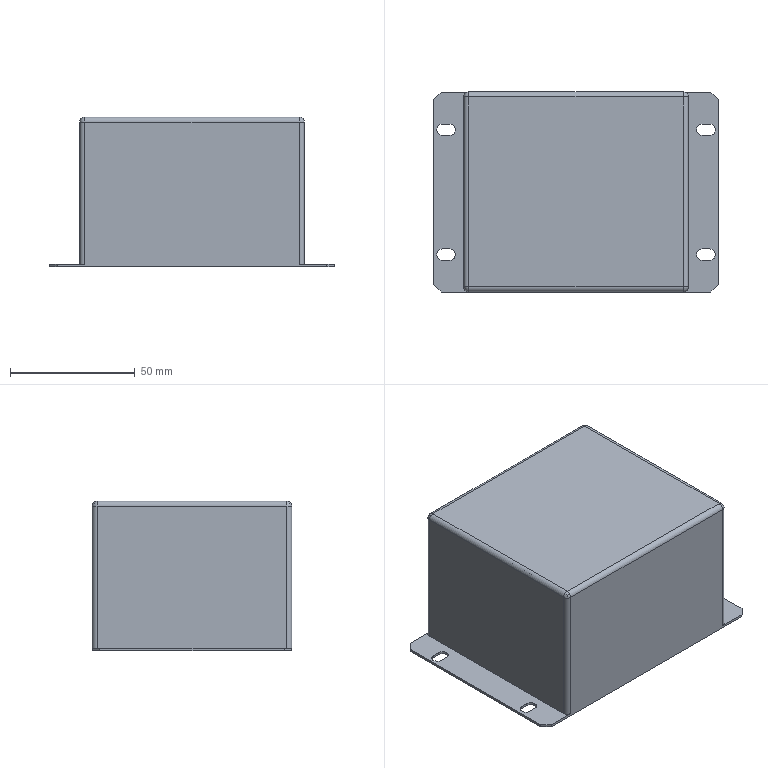Part | STEP file | 11-XJX-00311 | 1 solid | 51 faces | box 114 x 80 x 60 mm | volume 28319 mm3 | plane 27 | cylinder 20 | sphere 4 | commonest cylinder face diameters 4.5 x12 4 x8
STEP:
#1=CARTESIAN_POINT('',(55.75,-25.,0.));
#2=VERTEX_POINT('',#1);
#3=CARTESIAN_POINT('',(53.5,-22.75,0.));
#4=VERTEX_POINT('',#3);
#5=CARTESIAN_POINT('',(53.5,-25.,0.));
#6=DIRECTION('',(0.,0.,1.));
#7=DIRECTION('',(-1.,0.,0.));
#8=AXIS2_PLACEMENT_3D('',#5,#6,#7);
#9=CIRCLE('',#8,2.25);
#10=EDGE_CURVE('',#2,#4,#9,.T.);
#11=ORIENTED_EDGE('',*,*,#10,.F.);
#12=CARTESIAN_POINT('',(55.75,-25.,1.));
#13=VERTEX_POINT('',#12);
#14=CARTESIAN_POINT('',(55.75,-25.,0.));
#15=DIRECTION('',(0.,0.,1.));
#16=VECTOR('',#15,1000.);
#17=LINE('',#14,#16);
#18=EDGE_CURVE('',#2,#13,#17,.T.);
#19=ORIENTED_EDGE('',*,*,#18,.T.);
#20=CARTESIAN_POINT('',(53.5,-22.75,1.));
#21=VERTEX_POINT('',#20);
#22=CARTESIAN_POINT('',(53.5,-25.,1.));
#23=DIRECTION('',(0.,0.,1.));
#24=DIRECTION('',(-1.,0.,0.));
#25=AXIS2_PLACEMENT_3D('',#22,#23,#24);
#26=CIRCLE('',#25,2.25);
#27=EDGE_CURVE('',#13,#21,#26,.T.);
#28=ORIENTED_EDGE('',*,*,#27,.T.);
#29=CARTESIAN_POINT('',(53.5,-22.75,0.));
#30=DIRECTION('',(0.,0.,1.));
#31=VECTOR('',#30,1000.);
#32=LINE('',#29,#31);
#33=EDGE_CURVE('',#4,#21,#32,.T.);
#34=ORIENTED_EDGE('',*,*,#33,.F.);
#35=EDGE_LOOP('',(#11,#19,#28,#34));
#36=FACE_OUTER_BOUND('',#35,.T.);
#37=CARTESIAN_POINT('',(53.5,-25.,0.));
#38=DIRECTION('',(0.,0.,1.));
#39=DIRECTION('',(1.,0.,0.));
#40=AXIS2_PLACEMENT_3D('',#37,#38,#39);
#41=CYLINDRICAL_SURFACE('',#40,2.25);
#42=ADVANCED_FACE('',(#36),#41,.F.);
#43=CARTESIAN_POINT('',(-48.25,25.,0.));
#44=VERTEX_POINT('',#43);
#45=CARTESIAN_POINT('',(-50.5,27.25,0.));
#46=VERTEX_POINT('',#45);
#47=CARTESIAN_POINT('',(-50.5,25.,0.));
#48=DIRECTION('',(0.,0.,1.));
#49=DIRECTION('',(-1.,0.,0.));
#50=AXIS2_PLACEMENT_3D('',#47,#48,#49);
#51=CIRCLE('',#50,2.25);
#52=EDGE_CURVE('',#44,#46,#51,.T.);
#53=ORIENTED_EDGE('',*,*,#52,.F.);
#54=CARTESIAN_POINT('',(-48.25,25.,1.));
#55=VERTEX_POINT('',#54);
#56=CARTESIAN_POINT('',(-48.25,25.,0.));
#57=DIRECTION('',(0.,0.,1.));
#58=VECTOR('',#57,1000.);
#59=LINE('',#56,#58);
#60=EDGE_CURVE('',#44,#55,#59,.T.);
#61=ORIENTED_EDGE('',*,*,#60,.T.);
#62=CARTESIAN_POINT('',(-50.5,27.25,1.));
#63=VERTEX_POINT('',#62);
#64=CARTESIAN_POINT('',(-50.5,25.,1.));
#65=DIRECTION('',(0.,0.,1.));
#66=DIRECTION('',(-1.,0.,0.));
#67=AXIS2_PLACEMENT_3D('',#64,#65,#66);
#68=CIRCLE('',#67,2.25);
#69=EDGE_CURVE('',#55,#63,#68,.T.);
#70=ORIENTED_EDGE('',*,*,#69,.T.);
#71=CARTESIAN_POINT('',(-50.5,27.25,0.));
#72=DIRECTION('',(0.,0.,1.));
#73=VECTOR('',#72,1000.);
#74=LINE('',#71,#73);
#75=EDGE_CURVE('',#46,#63,#74,.T.);
#76=ORIENTED_EDGE('',*,*,#75,.F.);
#77=EDGE_LOOP('',(#53,#61,#70,#76));
#78=FACE_OUTER_BOUND('',#77,.T.);
#79=CARTESIAN_POINT('',(-50.5,25.,0.));
#80=DIRECTION('',(0.,0.,1.));
#81=DIRECTION('',(1.,0.,0.));
#82=AXIS2_PLACEMENT_3D('',#79,#80,#81);
#83=CYLINDRICAL_SURFACE('',#82,2.25);
#84=ADVANCED_FACE('',(#78),#83,.F.);
#85=CARTESIAN_POINT('',(-48.25,-25.,0.));
#86=VERTEX_POINT('',#85);
#87=CARTESIAN_POINT('',(-50.5,-22.75,0.));
#88=VERTEX_POINT('',#87);
#89=CARTESIAN_POINT('',(-50.5,-25.,0.));
#90=DIRECTION('',(0.,0.,1.));
#91=DIRECTION('',(1.,0.,0.));
#92=AXIS2_PLACEMENT_3D('',#89,#90,#91);
#93=CIRCLE('',#92,2.25);
#94=EDGE_CURVE('',#86,#88,#93,.T.);
#95=ORIENTED_EDGE('',*,*,#94,.F.);
#96=CARTESIAN_POINT('',(-48.25,-25.,1.));
#97=VERTEX_POINT('',#96);
#98=CARTESIAN_POINT('',(-48.25,-25.,0.));
#99=DIRECTION('',(0.,0.,1.));
#100=VECTOR('',#99,1000.);
#101=LINE('',#98,#100);
#102=EDGE_CURVE('',#86,#97,#101,.T.);
#103=ORIENTED_EDGE('',*,*,#102,.T.);
#104=CARTESIAN_POINT('',(-50.5,-22.75,1.));
#105=VERTEX_POINT('',#104);
#106=CARTESIAN_POINT('',(-50.5,-25.,1.));
#107=DIRECTION('',(0.,0.,1.));
#108=DIRECTION('',(1.,0.,0.));
#109=AXIS2_PLACEMENT_3D('',#106,#107,#108);
#110=CIRCLE('',#109,2.25);
#111=EDGE_CURVE('',#97,#105,#110,.T.);
#112=ORIENTED_EDGE('',*,*,#111,.T.);
#113=CARTESIAN_POINT('',(-50.5,-22.75,0.));
#114=DIRECTION('',(0.,0.,1.));
#115=VECTOR('',#114,1000.);
#116=LINE('',#113,#115);
#117=EDGE_CURVE('',#88,#105,#116,.T.);
#118=ORIENTED_EDGE('',*,*,#117,.F.);
#119=EDGE_LOOP('',(#95,#103,#112,#118));
#120=FACE_OUTER_BOUND('',#119,.T.);
#121=CARTESIAN_POINT('',(-50.5,-25.,0.));
#122=DIRECTION('',(0.,0.,1.));
#123=DIRECTION('',(1.,0.,0.));
#124=AXIS2_PLACEMENT_3D('',#121,#122,#123);
#125=CYLINDRICAL_SURFACE('',#124,2.25);
#126=ADVANCED_FACE('',(#120),#125,.F.);
#127=CARTESIAN_POINT('',(55.75,25.,0.));
#128=VERTEX_POINT('',#127);
#129=CARTESIAN_POINT('',(53.5,27.25,0.));
#130=VERTEX_POINT('',#129);
#131=CARTESIAN_POINT('',(53.5,25.,0.));
#132=DIRECTION('',(0.,0.,1.));
#133=DIRECTION('',(1.,0.,0.));
#134=AXIS2_PLACEMENT_3D('',#131,#132,#133);
#135=CIRCLE('',#134,2.25);
#136=EDGE_CURVE('',#128,#130,#135,.T.);
#137=ORIENTED_EDGE('',*,*,#136,.F.);
#138=CARTESIAN_POINT('',(55.75,25.,1.));
#139=VERTEX_POINT('',#138);
#140=CARTESIAN_POINT('',(55.75,25.,0.));
#141=DIRECTION('',(0.,0.,1.));
#142=VECTOR('',#141,1000.);
#143=LINE('',#140,#142);
#144=EDGE_CURVE('',#128,#139,#143,.T.);
#145=ORIENTED_EDGE('',*,*,#144,.T.);
#146=CARTESIAN_POINT('',(53.5,27.25,1.));
#147=VERTEX_POINT('',#146);
#148=CARTESIAN_POINT('',(53.5,25.,1.));
#149=DIRECTION('',(0.,0.,1.));
#150=DIRECTION('',(1.,0.,0.));
#151=AXIS2_PLACEMENT_3D('',#148,#149,#150);
#152=CIRCLE('',#151,2.25);
#153=EDGE_CURVE('',#139,#147,#152,.T.);
#154=ORIENTED_EDGE('',*,*,#153,.T.);
#155=CARTESIAN_POINT('',(53.5,27.25,0.));
#156=DIRECTION('',(0.,0.,1.));
#157=VECTOR('',#156,1000.);
#158=LINE('',#155,#157);
#159=EDGE_CURVE('',#130,#147,#158,.T.);
#160=ORIENTED_EDGE('',*,*,#159,.F.);
#161=EDGE_LOOP('',(#137,#145,#154,#160));
#162=FACE_OUTER_BOUND('',#161,.T.);
#163=CARTESIAN_POINT('',(53.5,25.,0.));
#164=DIRECTION('',(0.,0.,1.));
#165=DIRECTION('',(1.,0.,0.));
#166=AXIS2_PLACEMENT_3D('',#163,#164,#165);
#167=CYLINDRICAL_SURFACE('',#166,2.25);
#168=ADVANCED_FACE('',(#162),#167,.F.);
#169=CARTESIAN_POINT('',(45.,38.,1.));
#170=VERTEX_POINT('',#169);
#171=CARTESIAN_POINT('',(45.,-38.,1.));
#172=VERTEX_POINT('',#171);
#173=CARTESIAN_POINT('',(45.,40.,1.));
#174=DIRECTION('',(0.,-1.,0.));
#175=VECTOR('',#174,1000.);
#176=LINE('',#173,#175);
#177=EDGE_CURVE('',#170,#172,#176,.T.);
#178=ORIENTED_EDGE('',*,*,#177,.F.);
#179=CARTESIAN_POINT('',(45.,38.,58.));
#180=VERTEX_POINT('',#179);
#181=CARTESIAN_POINT('',(45.,38.,60.));
#182=DIRECTION('',(0.,0.,1.));
#183=VECTOR('',#182,1000.);
#184=LINE('',#181,#183);
#185=EDGE_CURVE('',#170,#180,#184,.T.);
#186=ORIENTED_EDGE('',*,*,#185,.T.);
#187=CARTESIAN_POINT('',(45.,-38.,58.));
#188=VERTEX_POINT('',#187);
#189=CARTESIAN_POINT('',(45.,-40.,58.));
#190=DIRECTION('',(0.,-1.,0.));
#191=VECTOR('',#190,1000.);
#192=LINE('',#189,#191);
#193=EDGE_CURVE('',#180,#188,#192,.T.);
#194=ORIENTED_EDGE('',*,*,#193,.T.);
#195=CARTESIAN_POINT('',(45.,-38.,60.));
#196=DIRECTION('',(0.,0.,-1.));
#197=VECTOR('',#196,1000.);
#198=LINE('',#195,#197);
#199=EDGE_CURVE('',#188,#172,#198,.T.);
#200=ORIENTED_EDGE('',*,*,#199,.T.);
#201=EDGE_LOOP('',(#178,#186,#194,#200));
#202=FACE_OUTER_BOUND('',#201,.T.);
#203=CARTESIAN_POINT('',(45.,40.,60.));
#204=DIRECTION('',(-1.,0.,0.));
#205=DIRECTION('',(0.,-1.,0.));
#206=AXIS2_PLACEMENT_3D('',#203,#204,#205);
#207=PLANE('',#206);
#208=ADVANCED_FACE('',(#202),#207,.F.);
#209=CARTESIAN_POINT('',(-43.,40.,1.));
#210=VERTEX_POINT('',#209);
#211=CARTESIAN_POINT('',(-54.,40.,1.));
#212=VERTEX_POINT('',#211);
#213=CARTESIAN_POINT('',(-45.,40.,1.));
#214=DIRECTION('',(-1.,0.,0.));
#215=VECTOR('',#214,1000.);
#216=LINE('',#213,#215);
#217=EDGE_CURVE('',#210,#212,#216,.T.);
#218=ORIENTED_EDGE('',*,*,#217,.F.);
#219=CARTESIAN_POINT('',(-43.,40.,58.));
#220=VERTEX_POINT('',#219);
#221=CARTESIAN_POINT('',(-43.,40.,60.));
#222=DIRECTION('',(0.,0.,1.));
#223=VECTOR('',#222,1000.);
#224=LINE('',#221,#223);
#225=EDGE_CURVE('',#210,#220,#224,.T.);
#226=ORIENTED_EDGE('',*,*,#225,.T.);
#227=CARTESIAN_POINT('',(43.,40.,58.));
#228=VERTEX_POINT('',#227);
#229=CARTESIAN_POINT('',(45.,40.,58.));
#230=DIRECTION('',(1.,0.,0.));
#231=VECTOR('',#230,1000.);
#232=LINE('',#229,#231);
#233=EDGE_CURVE('',#220,#228,#232,.T.);
#234=ORIENTED_EDGE('',*,*,#233,.T.);
#235=CARTESIAN_POINT('',(43.,40.,1.));
#236=VERTEX_POINT('',#235);
#237=CARTESIAN_POINT('',(43.,40.,60.));
#238=DIRECTION('',(0.,0.,-1.));
#239=VECTOR('',#238,1000.);
#240=LINE('',#237,#239);
#241=EDGE_CURVE('',#228,#236,#240,.T.);
#242=ORIENTED_EDGE('',*,*,#241,.T.);
#243=CARTESIAN_POINT('',(54.,40.,1.));
#244=VERTEX_POINT('',#243);
#245=CARTESIAN_POINT('',(45.,40.,1.));
#246=DIRECTION('',(-1.,0.,0.));
#247=VECTOR('',#246,1000.);
#248=LINE('',#245,#247);
#249=EDGE_CURVE('',#244,#236,#248,.T.);
#250=ORIENTED_EDGE('',*,*,#249,.F.);
#251=CARTESIAN_POINT('',(54.,40.,0.));
#252=VERTEX_POINT('',#251);
#253=CARTESIAN_POINT('',(54.,40.,0.));
#254=DIRECTION('',(0.,0.,-1.));
#255=VECTOR('',#254,1000.);
#256=LINE('',#253,#255);
#257=EDGE_CURVE('',#244,#252,#256,.T.);
#258=ORIENTED_EDGE('',*,*,#257,.T.);
#259=CARTESIAN_POINT('',(-54.,40.,0.));
#260=VERTEX_POINT('',#259);
#261=CARTESIAN_POINT('',(-45.,40.,0.));
#262=DIRECTION('',(-1.,0.,0.));
#263=VECTOR('',#262,1000.);
#264=LINE('',#261,#263);
#265=EDGE_CURVE('',#252,#260,#264,.T.);
#266=ORIENTED_EDGE('',*,*,#265,.T.);
#267=CARTESIAN_POINT('',(-54.,40.,1.));
#268=DIRECTION('',(0.,0.,1.));
#269=VECTOR('',#268,1000.);
#270=LINE('',#267,#269);
#271=EDGE_CURVE('',#260,#212,#270,.T.);
#272=ORIENTED_EDGE('',*,*,#271,.T.);
#273=EDGE_LOOP('',(#218,#226,#234,#242,#250,#258,#266,#272));
#274=FACE_OUTER_BOUND('',#273,.T.);
#275=CARTESIAN_POINT('',(-45.,40.,60.));
#276=DIRECTION('',(0.,-1.,0.));
#277=DIRECTION('',(0.,0.,-1.));
#278=AXIS2_PLACEMENT_3D('',#275,#276,#277);
#279=PLANE('',#278);
#280=ADVANCED_FACE('',(#274),#279,.F.);
#281=CARTESIAN_POINT('',(-45.,-38.,58.));
#282=VERTEX_POINT('',#281);
#283=CARTESIAN_POINT('',(-45.,38.,58.));
#284=VERTEX_POINT('',#283);
#285=CARTESIAN_POINT('',(-45.,40.,58.));
#286=DIRECTION('',(0.,1.,0.));
#287=VECTOR('',#286,1000.);
#288=LINE('',#285,#287);
#289=EDGE_CURVE('',#282,#284,#288,.T.);
#290=ORIENTED_EDGE('',*,*,#289,.T.);
#291=CARTESIAN_POINT('',(-45.,38.,1.));
#292=VERTEX_POINT('',#291);
#293=CARTESIAN_POINT('',(-45.,38.,60.));
#294=DIRECTION('',(0.,0.,-1.));
#295=VECTOR('',#294,1000.);
#296=LINE('',#293,#295);
#297=EDGE_CURVE('',#284,#292,#296,.T.);
#298=ORIENTED_EDGE('',*,*,#297,.T.);
#299=CARTESIAN_POINT('',(-45.,-38.,1.));
#300=VERTEX_POINT('',#299);
#301=CARTESIAN_POINT('',(-45.,40.,1.));
#302=DIRECTION('',(0.,-1.,0.));
#303=VECTOR('',#302,1000.);
#304=LINE('',#301,#303);
#305=EDGE_CURVE('',#292,#300,#304,.T.);
#306=ORIENTED_EDGE('',*,*,#305,.T.);
#307=CARTESIAN_POINT('',(-45.,-38.,60.));
#308=DIRECTION('',(0.,0.,1.));
#309=VECTOR('',#308,1000.);
#310=LINE('',#307,#309);
#311=EDGE_CURVE('',#300,#282,#310,.T.);
#312=ORIENTED_EDGE('',*,*,#311,.T.);
#313=EDGE_LOOP('',(#290,#298,#306,#312));
#314=FACE_OUTER_BOUND('',#313,.T.);
#315=CARTESIAN_POINT('',(-45.,40.,60.));
#316=DIRECTION('',(1.,0.,0.));
#317=DIRECTION('',(0.,1.,0.));
#318=AXIS2_PLACEMENT_3D('',#315,#316,#317);
#319=PLANE('',#318);
#320=ADVANCED_FACE('',(#314),#319,.F.);
#321=CARTESIAN_POINT('',(54.,-40.,1.));
#322=VERTEX_POINT('',#321);
#323=CARTESIAN_POINT('',(43.,-40.,1.));
#324=VERTEX_POINT('',#323);
#325=CARTESIAN_POINT('',(45.,-40.,1.));
#326=DIRECTION('',(-1.,0.,0.));
#327=VECTOR('',#326,1000.);
#328=LINE('',#325,#327);
#329=EDGE_CURVE('',#322,#324,#328,.T.);
#330=ORIENTED_EDGE('',*,*,#329,.T.);
#331=CARTESIAN_POINT('',(43.,-40.,58.));
#332=VERTEX_POINT('',#331);
#333=CARTESIAN_POINT('',(43.,-40.,60.));
#334=DIRECTION('',(0.,0.,1.));
#335=VECTOR('',#334,1000.);
#336=LINE('',#333,#335);
#337=EDGE_CURVE('',#324,#332,#336,.T.);
#338=ORIENTED_EDGE('',*,*,#337,.T.);
#339=CARTESIAN_POINT('',(-43.,-40.,58.));
#340=VERTEX_POINT('',#339);
#341=CARTESIAN_POINT('',(-45.,-40.,58.));
#342=DIRECTION('',(-1.,0.,0.));
#343=VECTOR('',#342,1000.);
#344=LINE('',#341,#343);
#345=EDGE_CURVE('',#332,#340,#344,.T.);
#346=ORIENTED_EDGE('',*,*,#345,.T.);
#347=CARTESIAN_POINT('',(-43.,-40.,1.));
#348=VERTEX_POINT('',#347);
#349=CARTESIAN_POINT('',(-43.,-40.,60.));
#350=DIRECTION('',(0.,0.,-1.));
#351=VECTOR('',#350,1000.);
#352=LINE('',#349,#351);
#353=EDGE_CURVE('',#340,#348,#352,.T.);
#354=ORIENTED_EDGE('',*,*,#353,.T.);
#355=CARTESIAN_POINT('',(-54.,-40.,1.));
#356=VERTEX_POINT('',#355);
#357=CARTESIAN_POINT('',(-45.,-40.,1.));
#358=DIRECTION('',(-1.,0.,0.));
#359=VECTOR('',#358,1000.);
#360=LINE('',#357,#359);
#361=EDGE_CURVE('',#348,#356,#360,.T.);
#362=ORIENTED_EDGE('',*,*,#361,.T.);
#363=CARTESIAN_POINT('',(-54.,-40.,0.));
#364=VERTEX_POINT('',#363);
#365=CARTESIAN_POINT('',(-54.,-40.,0.));
#366=DIRECTION('',(0.,0.,-1.));
#367=VECTOR('',#366,1000.);
#368=LINE('',#365,#367);
#369=EDGE_CURVE('',#356,#364,#368,.T.);
#370=ORIENTED_EDGE('',*,*,#369,.T.);
#371=CARTESIAN_POINT('',(54.,-40.,0.));
#372=VERTEX_POINT('',#371);
#373=CARTESIAN_POINT('',(-45.,-40.,0.));
#374=DIRECTION('',(1.,0.,0.));
#375=VECTOR('',#374,1000.);
#376=LINE('',#373,#375);
#377=EDGE_CURVE('',#364,#372,#376,.T.);
#378=ORIENTED_EDGE('',*,*,#377,.T.);
#379=CARTESIAN_POINT('',(54.,-40.,1.));
#380=DIRECTION('',(0.,0.,1.));
#381=VECTOR('',#380,1000.);
#382=LINE('',#379,#381);
#383=EDGE_CURVE('',#372,#322,#382,.T.);
#384=ORIENTED_EDGE('',*,*,#383,.T.);
#385=EDGE_LOOP('',(#330,#338,#346,#354,#362,#370,#378,#384));
#386=FACE_OUTER_BOUND('',#385,.T.);
#387=CARTESIAN_POINT('',(-45.,-40.,60.));
#388=DIRECTION('',(0.,1.,0.));
#389=DIRECTION('',(0.,0.,1.));
#390=AXIS2_PLACEMENT_3D('',#387,#388,#389);
#391=PLANE('',#390);
#392=ADVANCED_FACE('',(#386),#391,.F.);
#393=CARTESIAN_POINT('',(-43.,38.,60.));
#394=VERTEX_POINT('',#393);
#395=CARTESIAN_POINT('',(-43.,-38.,60.));
#396=VERTEX_POINT('',#395);
#397=CARTESIAN_POINT('',(-43.,-40.,60.));
#398=DIRECTION('',(0.,-1.,0.));
#399=VECTOR('',#398,1000.);
#400=LINE('',#397,#399);
#401=EDGE_CURVE('',#394,#396,#400,.T.);
#402=ORIENTED_EDGE('',*,*,#401,.T.);
#403=CARTESIAN_POINT('',(43.,-38.,60.));
#404=VERTEX_POINT('',#403);
#405=CARTESIAN_POINT('',(45.,-38.,60.));
#406=DIRECTION('',(1.,0.,0.));
#407=VECTOR('',#406,1000.);
#408=LINE('',#405,#407);
#409=EDGE_CURVE('',#396,#404,#408,.T.);
#410=ORIENTED_EDGE('',*,*,#409,.T.);
#411=CARTESIAN_POINT('',(43.,38.,60.));
#412=VERTEX_POINT('',#411);
#413=CARTESIAN_POINT('',(43.,40.,60.));
#414=DIRECTION('',(0.,1.,0.));
#415=VECTOR('',#414,1000.);
#416=LINE('',#413,#415);
#417=EDGE_CURVE('',#404,#412,#416,.T.);
#418=ORIENTED_EDGE('',*,*,#417,.T.);
#419=CARTESIAN_POINT('',(-45.,38.,60.));
#420=DIRECTION('',(-1.,0.,0.));
#421=VECTOR('',#420,1000.);
#422=LINE('',#419,#421);
#423=EDGE_CURVE('',#412,#394,#422,.T.);
#424=ORIENTED_EDGE('',*,*,#423,.T.);
#425=EDGE_LOOP('',(#402,#410,#418,#424));
#426=FACE_OUTER_BOUND('',#425,.T.);
#427=CARTESIAN_POINT('',(0.,0.,60.));
#428=DIRECTION('',(0.,0.,1.));
#429=DIRECTION('',(1.,0.,0.));
#430=AXIS2_PLACEMENT_3D('',#427,#428,#429);
#431=PLANE('',#430);
#432=ADVANCED_FACE('',(#426),#431,.T.);
#433=CARTESIAN_POINT('',(50.5,-22.75,0.));
#434=VERTEX_POINT('',#433);
#435=CARTESIAN_POINT('',(50.5,-22.75,0.));
#436=DIRECTION('',(-1.,0.,0.));
#437=VECTOR('',#436,1000.);
#438=LINE('',#435,#437);
#439=EDGE_CURVE('',#4,#434,#438,.T.);
#440=ORIENTED_EDGE('',*,*,#439,.T.);
#441=CARTESIAN_POINT('',(50.5,-27.25,0.));
#442=VERTEX_POINT('',#441);
#443=CARTESIAN_POINT('',(50.5,-25.,0.));
#444=DIRECTION('',(0.,0.,1.));
#445=DIRECTION('',(-1.,0.,0.));
#446=AXIS2_PLACEMENT_3D('',#443,#444,#445);
#447=CIRCLE('',#446,2.25);
#448=EDGE_CURVE('',#434,#442,#447,.T.);
#449=ORIENTED_EDGE('',*,*,#448,.T.);
#450=CARTESIAN_POINT('',(53.5,-27.25,0.));
#451=VERTEX_POINT('',#450);
#452=CARTESIAN_POINT('',(50.5,-27.25,0.));
#453=DIRECTION('',(1.,0.,0.));
#454=VECTOR('',#453,1000.);
#455=LINE('',#452,#454);
#456=EDGE_CURVE('',#442,#451,#455,.T.);
#457=ORIENTED_EDGE('',*,*,#456,.T.);
#458=CARTESIAN_POINT('',(53.5,-25.,0.));
#459=DIRECTION('',(0.,0.,1.));
#460=DIRECTION('',(-1.,0.,0.));
#461=AXIS2_PLACEMENT_3D('',#458,#459,#460);
#462=CIRCLE('',#461,2.25);
#463=EDGE_CURVE('',#451,#2,#462,.T.);
#464=ORIENTED_EDGE('',*,*,#463,.T.);
#465=ORIENTED_EDGE('',*,*,#10,.T.);
#466=EDGE_LOOP('',(#440,#449,#457,#464,#465));
#467=FACE_BOUND('',#466,.T.);
#468=CARTESIAN_POINT('',(-53.5,22.75,0.));
#469=VERTEX_POINT('',#468);
#470=CARTESIAN_POINT('',(-50.5,22.75,0.));
#471=VERTEX_POINT('',#470);
#472=CARTESIAN_POINT('',(-50.5,22.75,0.));
#473=DIRECTION('',(1.,0.,0.));
#474=VECTOR('',#473,1000.);
#475=LINE('',#472,#474);
#476=EDGE_CURVE('',#469,#471,#475,.T.);
#477=ORIENTED_EDGE('',*,*,#476,.T.);
#478=CARTESIAN_POINT('',(-50.5,25.,0.));
#479=DIRECTION('',(0.,0.,1.));
#480=DIRECTION('',(-1.,0.,0.));
#481=AXIS2_PLACEMENT_3D('',#478,#479,#480);
#482=CIRCLE('',#481,2.25);
#483=EDGE_CURVE('',#471,#44,#482,.T.);
#484=ORIENTED_EDGE('',*,*,#483,.T.);
#485=ORIENTED_EDGE('',*,*,#52,.T.);
#486=CARTESIAN_POINT('',(-53.5,27.25,0.));
#487=VERTEX_POINT('',#486);
#488=CARTESIAN_POINT('',(-50.5,27.25,0.));
#489=DIRECTION('',(-1.,0.,0.));
#490=VECTOR('',#489,1000.);
#491=LINE('',#488,#490);
#492=EDGE_CURVE('',#46,#487,#491,.T.);
#493=ORIENTED_EDGE('',*,*,#492,.T.);
#494=CARTESIAN_POINT('',(-53.5,25.,0.));
#495=DIRECTION('',(0.,0.,1.));
#496=DIRECTION('',(-1.,0.,0.));
#497=AXIS2_PLACEMENT_3D('',#494,#495,#496);
#498=CIRCLE('',#497,2.25);
#499=EDGE_CURVE('',#487,#469,#498,.T.);
#500=ORIENTED_EDGE('',*,*,#499,.T.);
#501=EDGE_LOOP('',(#477,#484,#485,#493,#500));
#502=FACE_BOUND('',#501,.T.);
#503=CARTESIAN_POINT('',(-53.5,-27.25,0.));
#504=VERTEX_POINT('',#503);
#505=CARTESIAN_POINT('',(-50.5,-27.25,0.));
#506=VERTEX_POINT('',#505);
#507=CARTESIAN_POINT('',(-50.5,-27.25,0.));
#508=DIRECTION('',(1.,0.,0.));
#509=VECTOR('',#508,1000.);
#510=LINE('',#507,#509);
#511=EDGE_CURVE('',#504,#506,#510,.T.);
#512=ORIENTED_EDGE('',*,*,#511,.T.);
#513=CARTESIAN_POINT('',(-50.5,-25.,0.));
#514=DIRECTION('',(0.,0.,1.));
#515=DIRECTION('',(1.,0.,0.));
#516=AXIS2_PLACEMENT_3D('',#513,#514,#515);
#517=CIRCLE('',#516,2.25);
#518=EDGE_CURVE('',#506,#86,#517,.T.);
#519=ORIENTED_EDGE('',*,*,#518,.T.);
#520=ORIENTED_EDGE('',*,*,#94,.T.);
#521=CARTESIAN_POINT('',(-53.5,-22.75,0.));
#522=VERTEX_POINT('',#521);
#523=CARTESIAN_POINT('',(-50.5,-22.75,0.));
#524=DIRECTION('',(-1.,0.,0.));
#525=VECTOR('',#524,1000.);
#526=LINE('',#523,#525);
#527=EDGE_CURVE('',#88,#522,#526,.T.);
#528=ORIENTED_EDGE('',*,*,#527,.T.);
#529=CARTESIAN_POINT('',(-53.5,-25.,0.));
#530=DIRECTION('',(0.,0.,1.));
#531=DIRECTION('',(1.,0.,0.));
#532=AXIS2_PLACEMENT_3D('',#529,#530,#531);
#533=CIRCLE('',#532,2.25);
#534=EDGE_CURVE('',#522,#504,#533,.T.);
#535=ORIENTED_EDGE('',*,*,#534,.T.);
#536=EDGE_LOOP('',(#512,#519,#520,#528,#535));
#537=FACE_BOUND('',#536,.T.);
#538=CARTESIAN_POINT('',(50.5,27.25,0.));
#539=VERTEX_POINT('',#538);
#540=CARTESIAN_POINT('',(50.5,27.25,0.));
#541=DIRECTION('',(-1.,0.,0.));
#542=VECTOR('',#541,1000.);
#543=LINE('',#540,#542);
#544=EDGE_CURVE('',#130,#539,#543,.T.);
#545=ORIENTED_EDGE('',*,*,#544,.T.);
#546=CARTESIAN_POINT('',(50.5,22.75,0.));
#547=VERTEX_POINT('',#546);
#548=CARTESIAN_POINT('',(50.5,25.,0.));
#549=DIRECTION('',(0.,0.,1.));
#550=DIRECTION('',(1.,0.,0.));
#551=AXIS2_PLACEMENT_3D('',#548,#549,#550);
#552=CIRCLE('',#551,2.25);
#553=EDGE_CURVE('',#539,#547,#552,.T.);
#554=ORIENTED_EDGE('',*,*,#553,.T.);
#555=CARTESIAN_POINT('',(53.5,22.75,0.));
#556=VERTEX_POINT('',#555);
#557=CARTESIAN_POINT('',(50.5,22.75,0.));
#558=DIRECTION('',(1.,0.,0.));
#559=VECTOR('',#558,1000.);
#560=LINE('',#557,#559);
#561=EDGE_CURVE('',#547,#556,#560,.T.);
#562=ORIENTED_EDGE('',*,*,#561,.T.);
#563=CARTESIAN_POINT('',(53.5,25.,0.));
#564=DIRECTION('',(0.,0.,1.));
#565=DIRECTION('',(1.,0.,0.));
#566=AXIS2_PLACEMENT_3D('',#563,#564,#565);
#567=CIRCLE('',#566,2.25);
#568=EDGE_CURVE('',#556,#128,#567,.T.);
#569=ORIENTED_EDGE('',*,*,#568,.T.);
#570=ORIENTED_EDGE('',*,*,#136,.T.);
#571=EDGE_LOOP('',(#545,#554,#562,#569,#570));
#572=FACE_BOUND('',#571,.T.);
#573=CARTESIAN_POINT('',(-44.,-39.,0.));
#574=VERTEX_POINT('',#573);
#575=CARTESIAN_POINT('',(44.,-39.,0.));
#576=VERTEX_POINT('',#575);
#577=CARTESIAN_POINT('',(-45.,-39.,0.));
#578=DIRECTION('',(1.,0.,0.));
#579=VECTOR('',#578,1000.);
#580=LINE('',#577,#579);
#581=EDGE_CURVE('',#574,#576,#580,.T.);
#582=ORIENTED_EDGE('',*,*,#581,.T.);
#583=CARTESIAN_POINT('',(44.,39.,0.));
#584=VERTEX_POINT('',#583);
#585=CARTESIAN_POINT('',(44.,40.,0.));
#586=DIRECTION('',(0.,1.,0.));
#587=VECTOR('',#586,1000.);
#588=LINE('',#585,#587);
#589=EDGE_CURVE('',#576,#584,#588,.T.);
#590=ORIENTED_EDGE('',*,*,#589,.T.);
#591=CARTESIAN_POINT('',(-44.,39.,0.));
#592=VERTEX_POINT('',#591);
#593=CARTESIAN_POINT('',(-45.,39.,0.));
#594=DIRECTION('',(-1.,0.,0.));
#595=VECTOR('',#594,1000.);
#596=LINE('',#593,#595);
#597=EDGE_CURVE('',#584,#592,#596,.T.);
#598=ORIENTED_EDGE('',*,*,#597,.T.);
#599=CARTESIAN_POINT('',(-44.,40.,0.));
#600=DIRECTION('',(0.,-1.,0.));
#601=VECTOR('',#600,1000.);
#602=LINE('',#599,#601);
#603=EDGE_CURVE('',#592,#574,#602,.T.);
#604=ORIENTED_EDGE('',*,*,#603,.T.);
#605=EDGE_LOOP('',(#582,#590,#598,#604));
#606=FACE_BOUND('',#605,.T.);
#607=CARTESIAN_POINT('',(-57.,37.,0.));
#608=VERTEX_POINT('',#607);
#609=CARTESIAN_POINT('',(-57.,-37.,0.));
#610=VERTEX_POINT('',#609);
#611=CARTESIAN_POINT('',(-57.,40.,0.));
#612=DIRECTION('',(0.,-1.,0.));
#613=VECTOR('',#612,1000.);
#614=LINE('',#611,#613);
#615=EDGE_CURVE('',#608,#610,#614,.T.);
#616=ORIENTED_EDGE('',*,*,#615,.F.);
#617=CARTESIAN_POINT('',(-57.,37.,0.));
#618=DIRECTION('',(0.7071,0.7071,0.));
#619=VECTOR('',#618,1000.);
#620=LINE('',#617,#619);
#621=EDGE_CURVE('',#608,#260,#620,.T.);
#622=ORIENTED_EDGE('',*,*,#621,.T.);
#623=ORIENTED_EDGE('',*,*,#265,.F.);
#624=CARTESIAN_POINT('',(57.,37.,0.));
#625=VERTEX_POINT('',#624);
#626=CARTESIAN_POINT('',(57.,37.,0.));
#627=DIRECTION('',(0.7071,-0.7071,0.));
#628=VECTOR('',#627,1000.);
#629=LINE('',#626,#628);
#630=EDGE_CURVE('',#252,#625,#629,.T.);
#631=ORIENTED_EDGE('',*,*,#630,.T.);
#632=CARTESIAN_POINT('',(57.,-37.,0.));
#633=VERTEX_POINT('',#632);
#634=CARTESIAN_POINT('',(57.,40.,0.));
#635=DIRECTION('',(0.,-1.,0.));
#636=VECTOR('',#635,1000.);
#637=LINE('',#634,#636);
#638=EDGE_CURVE('',#625,#633,#637,.T.);
#639=ORIENTED_EDGE('',*,*,#638,.T.);
#640=CARTESIAN_POINT('',(54.,-40.,0.));
#641=DIRECTION('',(-0.7071,-0.7071,0.));
#642=VECTOR('',#641,1000.);
#643=LINE('',#640,#642);
#644=EDGE_CURVE('',#633,#372,#643,.T.);
#645=ORIENTED_EDGE('',*,*,#644,.T.);
#646=ORIENTED_EDGE('',*,*,#377,.F.);
#647=CARTESIAN_POINT('',(-54.,-40.,0.));
#648=DIRECTION('',(-0.7071,0.7071,0.));
#649=VECTOR('',#648,1000.);
#650=LINE('',#647,#649);
#651=EDGE_CURVE('',#364,#610,#650,.T.);
#652=ORIENTED_EDGE('',*,*,#651,.T.);
#653=EDGE_LOOP('',(#616,#622,#623,#631,#639,#645,#646,#652));
#654=FACE_OUTER_BOUND('',#653,.T.);
#655=CARTESIAN_POINT('',(0.,0.,0.));
#656=DIRECTION('',(0.,0.,1.));
#657=DIRECTION('',(1.,0.,0.));
#658=AXIS2_PLACEMENT_3D('',#655,#656,#657);
#659=PLANE('',#658);
#660=ADVANCED_FACE('',(#467,#502,#537,#572,#606,#654),#659,.F.);
#661=ORIENTED_EDGE('',*,*,#589,.F.);
#662=CARTESIAN_POINT('',(44.,-39.,59.));
#663=VERTEX_POINT('',#662);
#664=CARTESIAN_POINT('',(44.,-39.,60.));
#665=DIRECTION('',(0.,0.,-1.));
#666=VECTOR('',#665,1000.);
#667=LINE('',#664,#666);
#668=EDGE_CURVE('',#663,#576,#667,.T.);
#669=ORIENTED_EDGE('',*,*,#668,.F.);
#670=CARTESIAN_POINT('',(44.,39.,59.));
#671=VERTEX_POINT('',#670);
#672=CARTESIAN_POINT('',(44.,40.,59.));
#673=DIRECTION('',(0.,1.,0.));
#674=VECTOR('',#673,1000.);
#675=LINE('',#672,#674);
#676=EDGE_CURVE('',#663,#671,#675,.T.);
#677=ORIENTED_EDGE('',*,*,#676,.T.);
#678=CARTESIAN_POINT('',(44.,39.,60.));
#679=DIRECTION('',(0.,0.,-1.));
#680=VECTOR('',#679,1000.);
#681=LINE('',#678,#680);
#682=EDGE_CURVE('',#671,#584,#681,.T.);
#683=ORIENTED_EDGE('',*,*,#682,.T.);
#684=EDGE_LOOP('',(#661,#669,#677,#683));
#685=FACE_OUTER_BOUND('',#684,.T.);
#686=CARTESIAN_POINT('',(44.,40.,60.));
#687=DIRECTION('',(-1.,0.,0.));
#688=DIRECTION('',(0.,-1.,0.));
#689=AXIS2_PLACEMENT_3D('',#686,#687,#688);
#690=PLANE('',#689);
#691=ADVANCED_FACE('',(#685),#690,.T.);
#692=ORIENTED_EDGE('',*,*,#597,.F.);
#693=ORIENTED_EDGE('',*,*,#682,.F.);
#694=CARTESIAN_POINT('',(-44.,39.,59.));
#695=VERTEX_POINT('',#694);
#696=CARTESIAN_POINT('',(-45.,39.,59.));
#697=DIRECTION('',(-1.,0.,0.));
#698=VECTOR('',#697,1000.);
#699=LINE('',#696,#698);
#700=EDGE_CURVE('',#671,#695,#699,.T.);
#701=ORIENTED_EDGE('',*,*,#700,.T.);
#702=CARTESIAN_POINT('',(-44.,39.,60.));
#703=DIRECTION('',(0.,0.,-1.));
#704=VECTOR('',#703,1000.);
#705=LINE('',#702,#704);
#706=EDGE_CURVE('',#695,#592,#705,.T.);
#707=ORIENTED_EDGE('',*,*,#706,.T.);
#708=EDGE_LOOP('',(#692,#693,#701,#707));
#709=FACE_OUTER_BOUND('',#708,.T.);
#710=CARTESIAN_POINT('',(-45.,39.,60.));
#711=DIRECTION('',(0.,-1.,0.));
#712=DIRECTION('',(0.,0.,-1.));
#713=AXIS2_PLACEMENT_3D('',#710,#711,#712);
#714=PLANE('',#713);
#715=ADVANCED_FACE('',(#709),#714,.T.);
#716=ORIENTED_EDGE('',*,*,#603,.F.);
#717=ORIENTED_EDGE('',*,*,#706,.F.);
#718=CARTESIAN_POINT('',(-44.,-39.,59.));
#719=VERTEX_POINT('',#718);
#720=CARTESIAN_POINT('',(-44.,40.,59.));
#721=DIRECTION('',(0.,-1.,0.));
#722=VECTOR('',#721,1000.);
#723=LINE('',#720,#722);
#724=EDGE_CURVE('',#695,#719,#723,.T.);
#725=ORIENTED_EDGE('',*,*,#724,.T.);
#726=CARTESIAN_POINT('',(-44.,-39.,60.));
#727=DIRECTION('',(0.,0.,-1.));
#728=VECTOR('',#727,1000.);
#729=LINE('',#726,#728);
#730=EDGE_CURVE('',#719,#574,#729,.T.);
#731=ORIENTED_EDGE('',*,*,#730,.T.);
#732=EDGE_LOOP('',(#716,#717,#725,#731));
#733=FACE_OUTER_BOUND('',#732,.T.);
#734=CARTESIAN_POINT('',(-44.,40.,60.));
#735=DIRECTION('',(1.,0.,0.));
#736=DIRECTION('',(0.,1.,0.));
#737=AXIS2_PLACEMENT_3D('',#734,#735,#736);
#738=PLANE('',#737);
#739=ADVANCED_FACE('',(#733),#738,.T.);
#740=ORIENTED_EDGE('',*,*,#581,.F.);
#741=ORIENTED_EDGE('',*,*,#730,.F.);
#742=CARTESIAN_POINT('',(-45.,-39.,59.));
#743=DIRECTION('',(1.,0.,0.));
#744=VECTOR('',#743,1000.);
#745=LINE('',#742,#744);
#746=EDGE_CURVE('',#719,#663,#745,.T.);
#747=ORIENTED_EDGE('',*,*,#746,.T.);
#748=ORIENTED_EDGE('',*,*,#668,.T.);
#749=EDGE_LOOP('',(#740,#741,#747,#748));
#750=FACE_OUTER_BOUND('',#749,.T.);
#751=CARTESIAN_POINT('',(-45.,-39.,60.));
#752=DIRECTION('',(0.,1.,0.));
#753=DIRECTION('',(0.,0.,1.));
#754=AXIS2_PLACEMENT_3D('',#751,#752,#753);
#755=PLANE('',#754);
#756=ADVANCED_FACE('',(#750),#755,.T.);
#757=ORIENTED_EDGE('',*,*,#676,.F.);
#758=ORIENTED_EDGE('',*,*,#746,.F.);
#759=ORIENTED_EDGE('',*,*,#724,.F.);
#760=ORIENTED_EDGE('',*,*,#700,.F.);
#761=EDGE_LOOP('',(#757,#758,#759,#760));
#762=FACE_OUTER_BOUND('',#761,.T.);
#763=CARTESIAN_POINT('',(0.,0.,59.));
#764=DIRECTION('',(0.,0.,1.));
#765=DIRECTION('',(1.,0.,0.));
#766=AXIS2_PLACEMENT_3D('',#763,#764,#765);
#767=PLANE('',#766);
#768=ADVANCED_FACE('',(#762),#767,.F.);
#769=CARTESIAN_POINT('',(50.5,-22.75,1.));
#770=VERTEX_POINT('',#769);
#771=CARTESIAN_POINT('',(50.5,-27.25,1.));
#772=VERTEX_POINT('',#771);
#773=CARTESIAN_POINT('',(50.5,-25.,1.));
#774=DIRECTION('',(0.,0.,1.));
#775=DIRECTION('',(-1.,0.,0.));
#776=AXIS2_PLACEMENT_3D('',#773,#774,#775);
#777=CIRCLE('',#776,2.25);
#778=EDGE_CURVE('',#770,#772,#777,.T.);
#779=ORIENTED_EDGE('',*,*,#778,.F.);
#780=CARTESIAN_POINT('',(50.5,-22.75,1.));
#781=DIRECTION('',(-1.,0.,0.));
#782=VECTOR('',#781,1000.);
#783=LINE('',#780,#782);
#784=EDGE_CURVE('',#21,#770,#783,.T.);
#785=ORIENTED_EDGE('',*,*,#784,.F.);
#786=ORIENTED_EDGE('',*,*,#27,.F.);
#787=CARTESIAN_POINT('',(53.5,-27.25,1.));
#788=VERTEX_POINT('',#787);
#789=CARTESIAN_POINT('',(53.5,-25.,1.));
#790=DIRECTION('',(0.,0.,1.));
#791=DIRECTION('',(-1.,0.,0.));
#792=AXIS2_PLACEMENT_3D('',#789,#790,#791);
#793=CIRCLE('',#792,2.25);
#794=EDGE_CURVE('',#788,#13,#793,.T.);
#795=ORIENTED_EDGE('',*,*,#794,.F.);
#796=CARTESIAN_POINT('',(50.5,-27.25,1.));
#797=DIRECTION('',(1.,0.,0.));
#798=VECTOR('',#797,1000.);
#799=LINE('',#796,#798);
#800=EDGE_CURVE('',#772,#788,#799,.T.);
#801=ORIENTED_EDGE('',*,*,#800,.F.);
#802=EDGE_LOOP('',(#779,#785,#786,#795,#801));
#803=FACE_BOUND('',#802,.T.);
#804=CARTESIAN_POINT('',(50.5,27.25,1.));
#805=VERTEX_POINT('',#804);
#806=CARTESIAN_POINT('',(50.5,22.75,1.));
#807=VERTEX_POINT('',#806);
#808=CARTESIAN_POINT('',(50.5,25.,1.));
#809=DIRECTION('',(0.,0.,1.));
#810=DIRECTION('',(1.,0.,0.));
#811=AXIS2_PLACEMENT_3D('',#808,#809,#810);
#812=CIRCLE('',#811,2.25);
#813=EDGE_CURVE('',#805,#807,#812,.T.);
#814=ORIENTED_EDGE('',*,*,#813,.F.);
#815=CARTESIAN_POINT('',(50.5,27.25,1.));
#816=DIRECTION('',(-1.,0.,0.));
#817=VECTOR('',#816,1000.);
#818=LINE('',#815,#817);
#819=EDGE_CURVE('',#147,#805,#818,.T.);
#820=ORIENTED_EDGE('',*,*,#819,.F.);
#821=ORIENTED_EDGE('',*,*,#153,.F.);
#822=CARTESIAN_POINT('',(53.5,22.75,1.));
#823=VERTEX_POINT('',#822);
#824=CARTESIAN_POINT('',(53.5,25.,1.));
#825=DIRECTION('',(0.,0.,1.));
#826=DIRECTION('',(1.,0.,0.));
#827=AXIS2_PLACEMENT_3D('',#824,#825,#826);
#828=CIRCLE('',#827,2.25);
#829=EDGE_CURVE('',#823,#139,#828,.T.);
#830=ORIENTED_EDGE('',*,*,#829,.F.);
#831=CARTESIAN_POINT('',(50.5,22.75,1.));
#832=DIRECTION('',(1.,0.,0.));
#833=VECTOR('',#832,1000.);
#834=LINE('',#831,#833);
#835=EDGE_CURVE('',#807,#823,#834,.T.);
#836=ORIENTED_EDGE('',*,*,#835,.F.);
#837=EDGE_LOOP('',(#814,#820,#821,#830,#836));
#838=FACE_BOUND('',#837,.T.);
#839=CARTESIAN_POINT('',(57.,37.,1.));
#840=VERTEX_POINT('',#839);
#841=CARTESIAN_POINT('',(57.,-37.,1.));
#842=VERTEX_POINT('',#841);
#843=CARTESIAN_POINT('',(57.,40.,1.));
#844=DIRECTION('',(0.,-1.,0.));
#845=VECTOR('',#844,1000.);
#846=LINE('',#843,#845);
#847=EDGE_CURVE('',#840,#842,#846,.T.);
#848=ORIENTED_EDGE('',*,*,#847,.F.);
#849=CARTESIAN_POINT('',(49.5,44.5,1.));
#850=DIRECTION('',(-0.7071,0.7071,0.));
#851=VECTOR('',#850,1000.);
#852=LINE('',#849,#851);
#853=EDGE_CURVE('',#840,#244,#852,.T.);
#854=ORIENTED_EDGE('',*,*,#853,.T.);
#855=ORIENTED_EDGE('',*,*,#249,.T.);
#856=CARTESIAN_POINT('',(43.,38.,1.));
#857=DIRECTION('',(0.,0.,-1.));
#858=DIRECTION('',(1.,0.,0.));
#859=AXIS2_PLACEMENT_3D('',#856,#857,#858);
#860=CIRCLE('',#859,2.);
#861=EDGE_CURVE('',#236,#170,#860,.T.);
#862=ORIENTED_EDGE('',*,*,#861,.T.);
#863=ORIENTED_EDGE('',*,*,#177,.T.);
#864=CARTESIAN_POINT('',(43.,-38.,1.));
#865=DIRECTION('',(0.,0.,-1.));
#866=DIRECTION('',(1.,0.,0.));
#867=AXIS2_PLACEMENT_3D('',#864,#865,#866);
#868=CIRCLE('',#867,2.);
#869=EDGE_CURVE('',#172,#324,#868,.T.);
#870=ORIENTED_EDGE('',*,*,#869,.T.);
#871=ORIENTED_EDGE('',*,*,#329,.F.);
#872=CARTESIAN_POINT('',(89.5,-4.5,1.));
#873=DIRECTION('',(0.7071,0.7071,0.));
#874=VECTOR('',#873,1000.);
#875=LINE('',#872,#874);
#876=EDGE_CURVE('',#322,#842,#875,.T.);
#877=ORIENTED_EDGE('',*,*,#876,.T.);
#878=EDGE_LOOP('',(#848,#854,#855,#862,#863,#870,#871,#877));
#879=FACE_OUTER_BOUND('',#878,.T.);
#880=CARTESIAN_POINT('',(45.,40.,1.));
#881=DIRECTION('',(0.,0.,1.));
#882=DIRECTION('',(1.,0.,0.));
#883=AXIS2_PLACEMENT_3D('',#880,#881,#882);
#884=PLANE('',#883);
#885=ADVANCED_FACE('',(#803,#838,#879),#884,.T.);
#886=ORIENTED_EDGE('',*,*,#638,.F.);
#887=CARTESIAN_POINT('',(57.,37.,1.));
#888=DIRECTION('',(0.,0.,1.));
#889=VECTOR('',#888,1000.);
#890=LINE('',#887,#889);
#891=EDGE_CURVE('',#625,#840,#890,.T.);
#892=ORIENTED_EDGE('',*,*,#891,.T.);
#893=ORIENTED_EDGE('',*,*,#847,.T.);
#894=CARTESIAN_POINT('',(57.,-37.,0.));
#895=DIRECTION('',(0.,0.,-1.));
#896=VECTOR('',#895,1000.);
#897=LINE('',#894,#896);
#898=EDGE_CURVE('',#842,#633,#897,.T.);
#899=ORIENTED_EDGE('',*,*,#898,.T.);
#900=EDGE_LOOP('',(#886,#892,#893,#899));
#901=FACE_OUTER_BOUND('',#900,.T.);
#902=CARTESIAN_POINT('',(57.,40.,0.));
#903=DIRECTION('',(1.,0.,0.));
#904=DIRECTION('',(0.,0.,-1.));
#905=AXIS2_PLACEMENT_3D('',#902,#903,#904);
#906=PLANE('',#905);
#907=ADVANCED_FACE('',(#901),#906,.T.);
#908=CARTESIAN_POINT('',(-57.,37.,1.));
#909=VERTEX_POINT('',#908);
#910=CARTESIAN_POINT('',(-57.,-37.,1.));
#911=VERTEX_POINT('',#910);
#912=CARTESIAN_POINT('',(-57.,40.,1.));
#913=DIRECTION('',(0.,-1.,0.));
#914=VECTOR('',#913,1000.);
#915=LINE('',#912,#914);
#916=EDGE_CURVE('',#909,#911,#915,.T.);
#917=ORIENTED_EDGE('',*,*,#916,.F.);
#918=CARTESIAN_POINT('',(-57.,37.,0.));
#919=DIRECTION('',(0.,0.,-1.));
#920=VECTOR('',#919,1000.);
#921=LINE('',#918,#920);
#922=EDGE_CURVE('',#909,#608,#921,.T.);
#923=ORIENTED_EDGE('',*,*,#922,.T.);
#924=ORIENTED_EDGE('',*,*,#615,.T.);
#925=CARTESIAN_POINT('',(-57.,-37.,1.));
#926=DIRECTION('',(0.,0.,1.));
#927=VECTOR('',#926,1000.);
#928=LINE('',#925,#927);
#929=EDGE_CURVE('',#610,#911,#928,.T.);
#930=ORIENTED_EDGE('',*,*,#929,.T.);
#931=EDGE_LOOP('',(#917,#923,#924,#930));
#932=FACE_OUTER_BOUND('',#931,.T.);
#933=CARTESIAN_POINT('',(-57.,40.,0.));
#934=DIRECTION('',(-1.,0.,0.));
#935=DIRECTION('',(0.,0.,1.));
#936=AXIS2_PLACEMENT_3D('',#933,#934,#935);
#937=PLANE('',#936);
#938=ADVANCED_FACE('',(#932),#937,.T.);
#939=CARTESIAN_POINT('',(-50.5,22.75,1.));
#940=VERTEX_POINT('',#939);
#941=CARTESIAN_POINT('',(-50.5,25.,1.));
#942=DIRECTION('',(0.,0.,1.));
#943=DIRECTION('',(-1.,0.,0.));
#944=AXIS2_PLACEMENT_3D('',#941,#942,#943);
#945=CIRCLE('',#944,2.25);
#946=EDGE_CURVE('',#940,#55,#945,.T.);
#947=ORIENTED_EDGE('',*,*,#946,.F.);
#948=CARTESIAN_POINT('',(-53.5,22.75,1.));
#949=VERTEX_POINT('',#948);
#950=CARTESIAN_POINT('',(-50.5,22.75,1.));
#951=DIRECTION('',(1.,0.,0.));
#952=VECTOR('',#951,1000.);
#953=LINE('',#950,#952);
#954=EDGE_CURVE('',#949,#940,#953,.T.);
#955=ORIENTED_EDGE('',*,*,#954,.F.);
#956=CARTESIAN_POINT('',(-53.5,27.25,1.));
#957=VERTEX_POINT('',#956);
#958=CARTESIAN_POINT('',(-53.5,25.,1.));
#959=DIRECTION('',(0.,0.,1.));
#960=DIRECTION('',(-1.,0.,0.));
#961=AXIS2_PLACEMENT_3D('',#958,#959,#960);
#962=CIRCLE('',#961,2.25);
#963=EDGE_CURVE('',#957,#949,#962,.T.);
#964=ORIENTED_EDGE('',*,*,#963,.F.);
#965=CARTESIAN_POINT('',(-50.5,27.25,1.));
#966=DIRECTION('',(-1.,0.,0.));
#967=VECTOR('',#966,1000.);
#968=LINE('',#965,#967);
#969=EDGE_CURVE('',#63,#957,#968,.T.);
#970=ORIENTED_EDGE('',*,*,#969,.F.);
#971=ORIENTED_EDGE('',*,*,#69,.F.);
#972=EDGE_LOOP('',(#947,#955,#964,#970,#971));
#973=FACE_BOUND('',#972,.T.);
#974=CARTESIAN_POINT('',(-50.5,-27.25,1.));
#975=VERTEX_POINT('',#974);
#976=CARTESIAN_POINT('',(-50.5,-25.,1.));
#977=DIRECTION('',(0.,0.,1.));
#978=DIRECTION('',(1.,0.,0.));
#979=AXIS2_PLACEMENT_3D('',#976,#977,#978);
#980=CIRCLE('',#979,2.25);
#981=EDGE_CURVE('',#975,#97,#980,.T.);
#982=ORIENTED_EDGE('',*,*,#981,.F.);
#983=CARTESIAN_POINT('',(-53.5,-27.25,1.));
#984=VERTEX_POINT('',#983);
#985=CARTESIAN_POINT('',(-50.5,-27.25,1.));
#986=DIRECTION('',(1.,0.,0.));
#987=VECTOR('',#986,1000.);
#988=LINE('',#985,#987);
#989=EDGE_CURVE('',#984,#975,#988,.T.);
#990=ORIENTED_EDGE('',*,*,#989,.F.);
#991=CARTESIAN_POINT('',(-53.5,-22.75,1.));
#992=VERTEX_POINT('',#991);
#993=CARTESIAN_POINT('',(-53.5,-25.,1.));
#994=DIRECTION('',(0.,0.,1.));
#995=DIRECTION('',(1.,0.,0.));
#996=AXIS2_PLACEMENT_3D('',#993,#994,#995);
#997=CIRCLE('',#996,2.25);
#998=EDGE_CURVE('',#992,#984,#997,.T.);
#999=ORIENTED_EDGE('',*,*,#998,.F.);
#1000=CARTESIAN_POINT('',(-50.5,-22.75,1.));
#1001=DIRECTION('',(-1.,0.,0.));
#1002=VECTOR('',#1001,1000.);
#1003=LINE('',#1000,#1002);
#1004=EDGE_CURVE('',#105,#992,#1003,.T.);
#1005=ORIENTED_EDGE('',*,*,#1004,.F.);
#1006=ORIENTED_EDGE('',*,*,#111,.F.);
#1007=EDGE_LOOP('',(#982,#990,#999,#1005,#1006));
#1008=FACE_BOUND('',#1007,.T.);
#1009=ORIENTED_EDGE('',*,*,#217,.T.);
#1010=CARTESIAN_POINT('',(-49.5,44.5,1.));
#1011=DIRECTION('',(-0.7071,-0.7071,0.));
#1012=VECTOR('',#1011,1000.);
#1013=LINE('',#1010,#1012);
#1014=EDGE_CURVE('',#212,#909,#1013,.T.);
#1015=ORIENTED_EDGE('',*,*,#1014,.T.);
#1016=ORIENTED_EDGE('',*,*,#916,.T.);
#1017=CARTESIAN_POINT('',(-89.5,-4.5,1.));
#1018=DIRECTION('',(0.7071,-0.7071,0.));
#1019=VECTOR('',#1018,1000.);
#1020=LINE('',#1017,#1019);
#1021=EDGE_CURVE('',#911,#356,#1020,.T.);
#1022=ORIENTED_EDGE('',*,*,#1021,.T.);
#1023=ORIENTED_EDGE('',*,*,#361,.F.);
#1024=CARTESIAN_POINT('',(-43.,-38.,1.));
#1025=DIRECTION('',(0.,0.,-1.));
#1026=DIRECTION('',(1.,0.,0.));
#1027=AXIS2_PLACEMENT_3D('',#1024,#1025,#1026);
#1028=CIRCLE('',#1027,2.);
#1029=EDGE_CURVE('',#348,#300,#1028,.T.);
#1030=ORIENTED_EDGE('',*,*,#1029,.T.);
#1031=ORIENTED_EDGE('',*,*,#305,.F.);
#1032=CARTESIAN_POINT('',(-43.,38.,1.));
#1033=DIRECTION('',(0.,0.,-1.));
#1034=DIRECTION('',(1.,0.,0.));
#1035=AXIS2_PLACEMENT_3D('',#1032,#1033,#1034);
#1036=CIRCLE('',#1035,2.);
#1037=EDGE_CURVE('',#292,#210,#1036,.T.);
#1038=ORIENTED_EDGE('',*,*,#1037,.T.);
#1039=EDGE_LOOP('',(#1009,#1015,#1016,#1022,#1023,#1030,#1031,#1038));
#1040=FACE_OUTER_BOUND('',#1039,.T.);
#1041=CARTESIAN_POINT('',(-45.,40.,1.));
#1042=DIRECTION('',(0.,0.,1.));
#1043=DIRECTION('',(1.,0.,0.));
#1044=AXIS2_PLACEMENT_3D('',#1041,#1042,#1043);
#1045=PLANE('',#1044);
#1046=ADVANCED_FACE('',(#973,#1008,#1040),#1045,.T.);
#1047=ORIENTED_EDGE('',*,*,#813,.T.);
#1048=CARTESIAN_POINT('',(50.5,22.75,0.));
#1049=DIRECTION('',(0.,0.,1.));
#1050=VECTOR('',#1049,1000.);
#1051=LINE('',#1048,#1050);
#1052=EDGE_CURVE('',#547,#807,#1051,.T.);
#1053=ORIENTED_EDGE('',*,*,#1052,.F.);
#1054=ORIENTED_EDGE('',*,*,#553,.F.);
#1055=CARTESIAN_POINT('',(50.5,27.25,0.));
#1056=DIRECTION('',(0.,0.,1.));
#1057=VECTOR('',#1056,1000.);
#1058=LINE('',#1055,#1057);
#1059=EDGE_CURVE('',#539,#805,#1058,.T.);
#1060=ORIENTED_EDGE('',*,*,#1059,.T.);
#1061=EDGE_LOOP('',(#1047,#1053,#1054,#1060));
#1062=FACE_OUTER_BOUND('',#1061,.T.);
#1063=CARTESIAN_POINT('',(50.5,25.,0.));
#1064=DIRECTION('',(0.,0.,1.));
#1065=DIRECTION('',(1.,0.,0.));
#1066=AXIS2_PLACEMENT_3D('',#1063,#1064,#1065);
#1067=CYLINDRICAL_SURFACE('',#1066,2.25);
#1068=ADVANCED_FACE('',(#1062),#1067,.F.);
#1069=ORIENTED_EDGE('',*,*,#819,.T.);
#1070=ORIENTED_EDGE('',*,*,#1059,.F.);
#1071=ORIENTED_EDGE('',*,*,#544,.F.);
#1072=ORIENTED_EDGE('',*,*,#159,.T.);
#1073=EDGE_LOOP('',(#1069,#1070,#1071,#1072));
#1074=FACE_OUTER_BOUND('',#1073,.T.);
#1075=CARTESIAN_POINT('',(50.5,27.25,0.));
#1076=DIRECTION('',(0.,1.,0.));
#1077=DIRECTION('',(0.,0.,1.));
#1078=AXIS2_PLACEMENT_3D('',#1075,#1076,#1077);
#1079=PLANE('',#1078);
#1080=ADVANCED_FACE('',(#1074),#1079,.F.);
#1081=ORIENTED_EDGE('',*,*,#144,.F.);
#1082=ORIENTED_EDGE('',*,*,#568,.F.);
#1083=CARTESIAN_POINT('',(53.5,22.75,0.));
#1084=DIRECTION('',(0.,0.,1.));
#1085=VECTOR('',#1084,1000.);
#1086=LINE('',#1083,#1085);
#1087=EDGE_CURVE('',#556,#823,#1086,.T.);
#1088=ORIENTED_EDGE('',*,*,#1087,.T.);
#1089=ORIENTED_EDGE('',*,*,#829,.T.);
#1090=EDGE_LOOP('',(#1081,#1082,#1088,#1089));
#1091=FACE_OUTER_BOUND('',#1090,.T.);
#1092=CARTESIAN_POINT('',(53.5,25.,0.));
#1093=DIRECTION('',(0.,0.,1.));
#1094=DIRECTION('',(1.,0.,0.));
#1095=AXIS2_PLACEMENT_3D('',#1092,#1093,#1094);
#1096=CYLINDRICAL_SURFACE('',#1095,2.25);
#1097=ADVANCED_FACE('',(#1091),#1096,.F.);
#1098=ORIENTED_EDGE('',*,*,#835,.T.);
#1099=ORIENTED_EDGE('',*,*,#1087,.F.);
#1100=ORIENTED_EDGE('',*,*,#561,.F.);
#1101=ORIENTED_EDGE('',*,*,#1052,.T.);
#1102=EDGE_LOOP('',(#1098,#1099,#1100,#1101));
#1103=FACE_OUTER_BOUND('',#1102,.T.);
#1104=CARTESIAN_POINT('',(50.5,22.75,0.));
#1105=DIRECTION('',(0.,-1.,0.));
#1106=DIRECTION('',(0.,0.,-1.));
#1107=AXIS2_PLACEMENT_3D('',#1104,#1105,#1106);
#1108=PLANE('',#1107);
#1109=ADVANCED_FACE('',(#1103),#1108,.F.);
#1110=ORIENTED_EDGE('',*,*,#102,.F.);
#1111=ORIENTED_EDGE('',*,*,#518,.F.);
#1112=CARTESIAN_POINT('',(-50.5,-27.25,0.));
#1113=DIRECTION('',(0.,0.,1.));
#1114=VECTOR('',#1113,1000.);
#1115=LINE('',#1112,#1114);
#1116=EDGE_CURVE('',#506,#975,#1115,.T.);
#1117=ORIENTED_EDGE('',*,*,#1116,.T.);
#1118=ORIENTED_EDGE('',*,*,#981,.T.);
#1119=EDGE_LOOP('',(#1110,#1111,#1117,#1118));
#1120=FACE_OUTER_BOUND('',#1119,.T.);
#1121=CARTESIAN_POINT('',(-50.5,-25.,0.));
#1122=DIRECTION('',(0.,0.,1.));
#1123=DIRECTION('',(1.,0.,0.));
#1124=AXIS2_PLACEMENT_3D('',#1121,#1122,#1123);
#1125=CYLINDRICAL_SURFACE('',#1124,2.25);
#1126=ADVANCED_FACE('',(#1120),#1125,.F.);
#1127=ORIENTED_EDGE('',*,*,#989,.T.);
#1128=ORIENTED_EDGE('',*,*,#1116,.F.);
#1129=ORIENTED_EDGE('',*,*,#511,.F.);
#1130=CARTESIAN_POINT('',(-53.5,-27.25,0.));
#1131=DIRECTION('',(0.,0.,1.));
#1132=VECTOR('',#1131,1000.);
#1133=LINE('',#1130,#1132);
#1134=EDGE_CURVE('',#504,#984,#1133,.T.);
#1135=ORIENTED_EDGE('',*,*,#1134,.T.);
#1136=EDGE_LOOP('',(#1127,#1128,#1129,#1135));
#1137=FACE_OUTER_BOUND('',#1136,.T.);
#1138=CARTESIAN_POINT('',(-50.5,-27.25,0.));
#1139=DIRECTION('',(0.,-1.,0.));
#1140=DIRECTION('',(0.,0.,-1.));
#1141=AXIS2_PLACEMENT_3D('',#1138,#1139,#1140);
#1142=PLANE('',#1141);
#1143=ADVANCED_FACE('',(#1137),#1142,.F.);
#1144=ORIENTED_EDGE('',*,*,#998,.T.);
#1145=ORIENTED_EDGE('',*,*,#1134,.F.);
#1146=ORIENTED_EDGE('',*,*,#534,.F.);
#1147=CARTESIAN_POINT('',(-53.5,-22.75,0.));
#1148=DIRECTION('',(0.,0.,1.));
#1149=VECTOR('',#1148,1000.);
#1150=LINE('',#1147,#1149);
#1151=EDGE_CURVE('',#522,#992,#1150,.T.);
#1152=ORIENTED_EDGE('',*,*,#1151,.T.);
#1153=EDGE_LOOP('',(#1144,#1145,#1146,#1152));
#1154=FACE_OUTER_BOUND('',#1153,.T.);
#1155=CARTESIAN_POINT('',(-53.5,-25.,0.));
#1156=DIRECTION('',(0.,0.,1.));
#1157=DIRECTION('',(1.,0.,0.));
#1158=AXIS2_PLACEMENT_3D('',#1155,#1156,#1157);
#1159=CYLINDRICAL_SURFACE('',#1158,2.25);
#1160=ADVANCED_FACE('',(#1154),#1159,.F.);
#1161=ORIENTED_EDGE('',*,*,#1004,.T.);
#1162=ORIENTED_EDGE('',*,*,#1151,.F.);
#1163=ORIENTED_EDGE('',*,*,#527,.F.);
#1164=ORIENTED_EDGE('',*,*,#117,.T.);
#1165=EDGE_LOOP('',(#1161,#1162,#1163,#1164));
#1166=FACE_OUTER_BOUND('',#1165,.T.);
#1167=CARTESIAN_POINT('',(-50.5,-22.75,0.));
#1168=DIRECTION('',(0.,1.,0.));
#1169=DIRECTION('',(0.,0.,1.));
#1170=AXIS2_PLACEMENT_3D('',#1167,#1168,#1169);
#1171=PLANE('',#1170);
#1172=ADVANCED_FACE('',(#1166),#1171,.F.);
#1173=ORIENTED_EDGE('',*,*,#60,.F.);
#1174=ORIENTED_EDGE('',*,*,#483,.F.);
#1175=CARTESIAN_POINT('',(-50.5,22.75,0.));
#1176=DIRECTION('',(0.,0.,1.));
#1177=VECTOR('',#1176,1000.);
#1178=LINE('',#1175,#1177);
#1179=EDGE_CURVE('',#471,#940,#1178,.T.);
#1180=ORIENTED_EDGE('',*,*,#1179,.T.);
#1181=ORIENTED_EDGE('',*,*,#946,.T.);
#1182=EDGE_LOOP('',(#1173,#1174,#1180,#1181));
#1183=FACE_OUTER_BOUND('',#1182,.T.);
#1184=CARTESIAN_POINT('',(-50.5,25.,0.));
#1185=DIRECTION('',(0.,0.,1.));
#1186=DIRECTION('',(1.,0.,0.));
#1187=AXIS2_PLACEMENT_3D('',#1184,#1185,#1186);
#1188=CYLINDRICAL_SURFACE('',#1187,2.25);
#1189=ADVANCED_FACE('',(#1183),#1188,.F.);
#1190=ORIENTED_EDGE('',*,*,#954,.T.);
#1191=ORIENTED_EDGE('',*,*,#1179,.F.);
#1192=ORIENTED_EDGE('',*,*,#476,.F.);
#1193=CARTESIAN_POINT('',(-53.5,22.75,0.));
#1194=DIRECTION('',(0.,0.,1.));
#1195=VECTOR('',#1194,1000.);
#1196=LINE('',#1193,#1195);
#1197=EDGE_CURVE('',#469,#949,#1196,.T.);
#1198=ORIENTED_EDGE('',*,*,#1197,.T.);
#1199=EDGE_LOOP('',(#1190,#1191,#1192,#1198));
#1200=FACE_OUTER_BOUND('',#1199,.T.);
#1201=CARTESIAN_POINT('',(-50.5,22.75,0.));
#1202=DIRECTION('',(0.,-1.,0.));
#1203=DIRECTION('',(0.,0.,-1.));
#1204=AXIS2_PLACEMENT_3D('',#1201,#1202,#1203);
#1205=PLANE('',#1204);
#1206=ADVANCED_FACE('',(#1200),#1205,.F.);
#1207=ORIENTED_EDGE('',*,*,#963,.T.);
#1208=ORIENTED_EDGE('',*,*,#1197,.F.);
#1209=ORIENTED_EDGE('',*,*,#499,.F.);
#1210=CARTESIAN_POINT('',(-53.5,27.25,0.));
#1211=DIRECTION('',(0.,0.,1.));
#1212=VECTOR('',#1211,1000.);
#1213=LINE('',#1210,#1212);
#1214=EDGE_CURVE('',#487,#957,#1213,.T.);
#1215=ORIENTED_EDGE('',*,*,#1214,.T.);
#1216=EDGE_LOOP('',(#1207,#1208,#1209,#1215));
#1217=FACE_OUTER_BOUND('',#1216,.T.);
#1218=CARTESIAN_POINT('',(-53.5,25.,0.));
#1219=DIRECTION('',(0.,0.,1.));
#1220=DIRECTION('',(1.,0.,0.));
#1221=AXIS2_PLACEMENT_3D('',#1218,#1219,#1220);
#1222=CYLINDRICAL_SURFACE('',#1221,2.25);
#1223=ADVANCED_FACE('',(#1217),#1222,.F.);
#1224=ORIENTED_EDGE('',*,*,#969,.T.);
#1225=ORIENTED_EDGE('',*,*,#1214,.F.);
#1226=ORIENTED_EDGE('',*,*,#492,.F.);
#1227=ORIENTED_EDGE('',*,*,#75,.T.);
#1228=EDGE_LOOP('',(#1224,#1225,#1226,#1227));
#1229=FACE_OUTER_BOUND('',#1228,.T.);
#1230=CARTESIAN_POINT('',(-50.5,27.25,0.));
#1231=DIRECTION('',(0.,1.,0.));
#1232=DIRECTION('',(0.,0.,1.));
#1233=AXIS2_PLACEMENT_3D('',#1230,#1231,#1232);
#1234=PLANE('',#1233);
#1235=ADVANCED_FACE('',(#1229),#1234,.F.);
#1236=ORIENTED_EDGE('',*,*,#778,.T.);
#1237=CARTESIAN_POINT('',(50.5,-27.25,0.));
#1238=DIRECTION('',(0.,0.,1.));
#1239=VECTOR('',#1238,1000.);
#1240=LINE('',#1237,#1239);
#1241=EDGE_CURVE('',#442,#772,#1240,.T.);
#1242=ORIENTED_EDGE('',*,*,#1241,.F.);
#1243=ORIENTED_EDGE('',*,*,#448,.F.);
#1244=CARTESIAN_POINT('',(50.5,-22.75,0.));
#1245=DIRECTION('',(0.,0.,1.));
#1246=VECTOR('',#1245,1000.);
#1247=LINE('',#1244,#1246);
#1248=EDGE_CURVE('',#434,#770,#1247,.T.);
#1249=ORIENTED_EDGE('',*,*,#1248,.T.);
#1250=EDGE_LOOP('',(#1236,#1242,#1243,#1249));
#1251=FACE_OUTER_BOUND('',#1250,.T.);
#1252=CARTESIAN_POINT('',(50.5,-25.,0.));
#1253=DIRECTION('',(0.,0.,1.));
#1254=DIRECTION('',(1.,0.,0.));
#1255=AXIS2_PLACEMENT_3D('',#1252,#1253,#1254);
#1256=CYLINDRICAL_SURFACE('',#1255,2.25);
#1257=ADVANCED_FACE('',(#1251),#1256,.F.);
#1258=ORIENTED_EDGE('',*,*,#784,.T.);
#1259=ORIENTED_EDGE('',*,*,#1248,.F.);
#1260=ORIENTED_EDGE('',*,*,#439,.F.);
#1261=ORIENTED_EDGE('',*,*,#33,.T.);
#1262=EDGE_LOOP('',(#1258,#1259,#1260,#1261));
#1263=FACE_OUTER_BOUND('',#1262,.T.);
#1264=CARTESIAN_POINT('',(50.5,-22.75,0.));
#1265=DIRECTION('',(0.,1.,0.));
#1266=DIRECTION('',(0.,0.,1.));
#1267=AXIS2_PLACEMENT_3D('',#1264,#1265,#1266);
#1268=PLANE('',#1267);
#1269=ADVANCED_FACE('',(#1263),#1268,.F.);
#1270=ORIENTED_EDGE('',*,*,#18,.F.);
#1271=ORIENTED_EDGE('',*,*,#463,.F.);
#1272=CARTESIAN_POINT('',(53.5,-27.25,0.));
#1273=DIRECTION('',(0.,0.,1.));
#1274=VECTOR('',#1273,1000.);
#1275=LINE('',#1272,#1274);
#1276=EDGE_CURVE('',#451,#788,#1275,.T.);
#1277=ORIENTED_EDGE('',*,*,#1276,.T.);
#1278=ORIENTED_EDGE('',*,*,#794,.T.);
#1279=EDGE_LOOP('',(#1270,#1271,#1277,#1278));
#1280=FACE_OUTER_BOUND('',#1279,.T.);
#1281=CARTESIAN_POINT('',(53.5,-25.,0.));
#1282=DIRECTION('',(0.,0.,1.));
#1283=DIRECTION('',(1.,0.,0.));
#1284=AXIS2_PLACEMENT_3D('',#1281,#1282,#1283);
#1285=CYLINDRICAL_SURFACE('',#1284,2.25);
#1286=ADVANCED_FACE('',(#1280),#1285,.F.);
#1287=ORIENTED_EDGE('',*,*,#800,.T.);
#1288=ORIENTED_EDGE('',*,*,#1276,.F.);
#1289=ORIENTED_EDGE('',*,*,#456,.F.);
#1290=ORIENTED_EDGE('',*,*,#1241,.T.);
#1291=EDGE_LOOP('',(#1287,#1288,#1289,#1290));
#1292=FACE_OUTER_BOUND('',#1291,.T.);
#1293=CARTESIAN_POINT('',(50.5,-27.25,0.));
#1294=DIRECTION('',(0.,-1.,0.));
#1295=DIRECTION('',(0.,0.,-1.));
#1296=AXIS2_PLACEMENT_3D('',#1293,#1294,#1295);
#1297=PLANE('',#1296);
#1298=ADVANCED_FACE('',(#1292),#1297,.F.);
#1299=ORIENTED_EDGE('',*,*,#1014,.F.);
#1300=ORIENTED_EDGE('',*,*,#271,.F.);
#1301=ORIENTED_EDGE('',*,*,#621,.F.);
#1302=ORIENTED_EDGE('',*,*,#922,.F.);
#1303=EDGE_LOOP('',(#1299,#1300,#1301,#1302));
#1304=FACE_OUTER_BOUND('',#1303,.T.);
#1305=CARTESIAN_POINT('',(-57.,37.,0.));
#1306=DIRECTION('',(-0.7071,0.7071,0.));
#1307=DIRECTION('',(0.,0.,1.));
#1308=AXIS2_PLACEMENT_3D('',#1305,#1306,#1307);
#1309=PLANE('',#1308);
#1310=ADVANCED_FACE('',(#1304),#1309,.T.);
#1311=ORIENTED_EDGE('',*,*,#1021,.F.);
#1312=ORIENTED_EDGE('',*,*,#929,.F.);
#1313=ORIENTED_EDGE('',*,*,#651,.F.);
#1314=ORIENTED_EDGE('',*,*,#369,.F.);
#1315=EDGE_LOOP('',(#1311,#1312,#1313,#1314));
#1316=FACE_OUTER_BOUND('',#1315,.T.);
#1317=CARTESIAN_POINT('',(-54.,-40.,60.));
#1318=DIRECTION('',(-0.7071,-0.7071,0.));
#1319=DIRECTION('',(0.,0.,1.));
#1320=AXIS2_PLACEMENT_3D('',#1317,#1318,#1319);
#1321=PLANE('',#1320);
#1322=ADVANCED_FACE('',(#1316),#1321,.T.);
#1323=ORIENTED_EDGE('',*,*,#630,.F.);
#1324=ORIENTED_EDGE('',*,*,#257,.F.);
#1325=ORIENTED_EDGE('',*,*,#853,.F.);
#1326=ORIENTED_EDGE('',*,*,#891,.F.);
#1327=EDGE_LOOP('',(#1323,#1324,#1325,#1326));
#1328=FACE_OUTER_BOUND('',#1327,.T.);
#1329=CARTESIAN_POINT('',(57.,37.,0.));
#1330=DIRECTION('',(0.7071,0.7071,0.));
#1331=DIRECTION('',(0.,0.,-1.));
#1332=AXIS2_PLACEMENT_3D('',#1329,#1330,#1331);
#1333=PLANE('',#1332);
#1334=ADVANCED_FACE('',(#1328),#1333,.T.);
#1335=ORIENTED_EDGE('',*,*,#644,.F.);
#1336=ORIENTED_EDGE('',*,*,#898,.F.);
#1337=ORIENTED_EDGE('',*,*,#876,.F.);
#1338=ORIENTED_EDGE('',*,*,#383,.F.);
#1339=EDGE_LOOP('',(#1335,#1336,#1337,#1338));
#1340=FACE_OUTER_BOUND('',#1339,.T.);
#1341=CARTESIAN_POINT('',(54.,-40.,60.));
#1342=DIRECTION('',(0.7071,-0.7071,0.));
#1343=DIRECTION('',(0.,0.,-1.));
#1344=AXIS2_PLACEMENT_3D('',#1341,#1342,#1343);
#1345=PLANE('',#1344);
#1346=ADVANCED_FACE('',(#1340),#1345,.T.);
#1347=ORIENTED_EDGE('',*,*,#1037,.F.);
#1348=ORIENTED_EDGE('',*,*,#297,.F.);
#1349=CARTESIAN_POINT('',(-43.,38.,58.));
#1350=DIRECTION('',(0.,0.,1.));
#1351=DIRECTION('',(1.,0.,0.));
#1352=AXIS2_PLACEMENT_3D('',#1349,#1350,#1351);
#1353=CIRCLE('',#1352,2.);
#1354=EDGE_CURVE('',#220,#284,#1353,.T.);
#1355=ORIENTED_EDGE('',*,*,#1354,.F.);
#1356=ORIENTED_EDGE('',*,*,#225,.F.);
#1357=EDGE_LOOP('',(#1347,#1348,#1355,#1356));
#1358=FACE_OUTER_BOUND('',#1357,.T.);
#1359=CARTESIAN_POINT('',(-43.,38.,60.));
#1360=DIRECTION('',(0.,0.,-1.));
#1361=DIRECTION('',(-1.,0.,0.));
#1362=AXIS2_PLACEMENT_3D('',#1359,#1360,#1361);
#1363=CYLINDRICAL_SURFACE('',#1362,2.);
#1364=ADVANCED_FACE('',(#1358),#1363,.T.);
#1365=CARTESIAN_POINT('',(43.,38.,58.));
#1366=DIRECTION('',(1.,0.,0.));
#1367=DIRECTION('',(0.,0.,-1.));
#1368=AXIS2_PLACEMENT_3D('',#1365,#1366,#1367);
#1369=CIRCLE('',#1368,2.);
#1370=EDGE_CURVE('',#228,#412,#1369,.T.);
#1371=ORIENTED_EDGE('',*,*,#1370,.F.);
#1372=ORIENTED_EDGE('',*,*,#233,.F.);
#1373=CARTESIAN_POINT('',(-43.,38.,58.));
#1374=DIRECTION('',(-1.,0.,0.));
#1375=DIRECTION('',(0.,0.,1.));
#1376=AXIS2_PLACEMENT_3D('',#1373,#1374,#1375);
#1377=CIRCLE('',#1376,2.);
#1378=EDGE_CURVE('',#394,#220,#1377,.T.);
#1379=ORIENTED_EDGE('',*,*,#1378,.F.);
#1380=ORIENTED_EDGE('',*,*,#423,.F.);
#1381=EDGE_LOOP('',(#1371,#1372,#1379,#1380));
#1382=FACE_OUTER_BOUND('',#1381,.T.);
#1383=CARTESIAN_POINT('',(0.,38.,58.));
#1384=DIRECTION('',(1.,0.,0.));
#1385=DIRECTION('',(0.,0.,-1.));
#1386=AXIS2_PLACEMENT_3D('',#1383,#1384,#1385);
#1387=CYLINDRICAL_SURFACE('',#1386,2.);
#1388=ADVANCED_FACE('',(#1382),#1387,.T.);
#1389=ORIENTED_EDGE('',*,*,#861,.F.);
#1390=ORIENTED_EDGE('',*,*,#241,.F.);
#1391=CARTESIAN_POINT('',(43.,38.,58.));
#1392=DIRECTION('',(0.,0.,1.));
#1393=DIRECTION('',(1.,0.,0.));
#1394=AXIS2_PLACEMENT_3D('',#1391,#1392,#1393);
#1395=CIRCLE('',#1394,2.);
#1396=EDGE_CURVE('',#180,#228,#1395,.T.);
#1397=ORIENTED_EDGE('',*,*,#1396,.F.);
#1398=ORIENTED_EDGE('',*,*,#185,.F.);
#1399=EDGE_LOOP('',(#1389,#1390,#1397,#1398));
#1400=FACE_OUTER_BOUND('',#1399,.T.);
#1401=CARTESIAN_POINT('',(43.,38.,60.));
#1402=DIRECTION('',(0.,0.,-1.));
#1403=DIRECTION('',(-1.,0.,0.));
#1404=AXIS2_PLACEMENT_3D('',#1401,#1402,#1403);
#1405=CYLINDRICAL_SURFACE('',#1404,2.);
#1406=ADVANCED_FACE('',(#1400),#1405,.T.);
#1407=ORIENTED_EDGE('',*,*,#1378,.T.);
#1408=ORIENTED_EDGE('',*,*,#1354,.T.);
#1409=CARTESIAN_POINT('',(-43.,38.,58.));
#1410=DIRECTION('',(0.,-1.,0.));
#1411=DIRECTION('',(0.,0.,1.));
#1412=AXIS2_PLACEMENT_3D('',#1409,#1410,#1411);
#1413=CIRCLE('',#1412,2.);
#1414=EDGE_CURVE('',#394,#284,#1413,.T.);
#1415=ORIENTED_EDGE('',*,*,#1414,.F.);
#1416=EDGE_LOOP('',(#1407,#1408,#1415));
#1417=FACE_OUTER_BOUND('',#1416,.T.);
#1418=CARTESIAN_POINT('',(-43.,38.,58.));
#1419=DIRECTION('',(0.,1.,0.));
#1420=DIRECTION('',(1.,0.,0.));
#1421=AXIS2_PLACEMENT_3D('',#1418,#1419,#1420);
#1422=SPHERICAL_SURFACE('',#1421,2.);
#1423=ADVANCED_FACE('',(#1417),#1422,.T.);
#1424=ORIENTED_EDGE('',*,*,#1396,.T.);
#1425=ORIENTED_EDGE('',*,*,#1370,.T.);
#1426=CARTESIAN_POINT('',(43.,38.,58.));
#1427=DIRECTION('',(0.,-1.,0.));
#1428=DIRECTION('',(0.,0.,1.));
#1429=AXIS2_PLACEMENT_3D('',#1426,#1427,#1428);
#1430=CIRCLE('',#1429,2.);
#1431=EDGE_CURVE('',#180,#412,#1430,.T.);
#1432=ORIENTED_EDGE('',*,*,#1431,.F.);
#1433=EDGE_LOOP('',(#1424,#1425,#1432));
#1434=FACE_OUTER_BOUND('',#1433,.T.);
#1435=CARTESIAN_POINT('',(43.,38.,58.));
#1436=DIRECTION('',(0.,1.,0.));
#1437=DIRECTION('',(1.,0.,0.));
#1438=AXIS2_PLACEMENT_3D('',#1435,#1436,#1437);
#1439=SPHERICAL_SURFACE('',#1438,2.);
#1440=ADVANCED_FACE('',(#1434),#1439,.T.);
#1441=ORIENTED_EDGE('',*,*,#1029,.F.);
#1442=ORIENTED_EDGE('',*,*,#353,.F.);
#1443=CARTESIAN_POINT('',(-43.,-38.,58.));
#1444=DIRECTION('',(0.,0.,1.));
#1445=DIRECTION('',(1.,0.,0.));
#1446=AXIS2_PLACEMENT_3D('',#1443,#1444,#1445);
#1447=CIRCLE('',#1446,2.);
#1448=EDGE_CURVE('',#282,#340,#1447,.T.);
#1449=ORIENTED_EDGE('',*,*,#1448,.F.);
#1450=ORIENTED_EDGE('',*,*,#311,.F.);
#1451=EDGE_LOOP('',(#1441,#1442,#1449,#1450));
#1452=FACE_OUTER_BOUND('',#1451,.T.);
#1453=CARTESIAN_POINT('',(-43.,-38.,60.));
#1454=DIRECTION('',(0.,0.,-1.));
#1455=DIRECTION('',(-1.,0.,0.));
#1456=AXIS2_PLACEMENT_3D('',#1453,#1454,#1455);
#1457=CYLINDRICAL_SURFACE('',#1456,2.);
#1458=ADVANCED_FACE('',(#1452),#1457,.T.);
#1459=ORIENTED_EDGE('',*,*,#1414,.T.);
#1460=ORIENTED_EDGE('',*,*,#289,.F.);
#1461=CARTESIAN_POINT('',(-43.,-38.,58.));
#1462=DIRECTION('',(0.,-1.,0.));
#1463=DIRECTION('',(0.,0.,-1.));
#1464=AXIS2_PLACEMENT_3D('',#1461,#1462,#1463);
#1465=CIRCLE('',#1464,2.);
#1466=EDGE_CURVE('',#396,#282,#1465,.T.);
#1467=ORIENTED_EDGE('',*,*,#1466,.F.);
#1468=ORIENTED_EDGE('',*,*,#401,.F.);
#1469=EDGE_LOOP('',(#1459,#1460,#1467,#1468));
#1470=FACE_OUTER_BOUND('',#1469,.T.);
#1471=CARTESIAN_POINT('',(-43.,0.,58.));
#1472=DIRECTION('',(0.,1.,0.));
#1473=DIRECTION('',(-1.,0.,0.));
#1474=AXIS2_PLACEMENT_3D('',#1471,#1472,#1473);
#1475=CYLINDRICAL_SURFACE('',#1474,2.);
#1476=ADVANCED_FACE('',(#1470),#1475,.T.);
#1477=ORIENTED_EDGE('',*,*,#1431,.T.);
#1478=ORIENTED_EDGE('',*,*,#417,.F.);
#1479=CARTESIAN_POINT('',(43.,-38.,58.));
#1480=DIRECTION('',(0.,-1.,0.));
#1481=DIRECTION('',(0.,0.,-1.));
#1482=AXIS2_PLACEMENT_3D('',#1479,#1480,#1481);
#1483=CIRCLE('',#1482,2.);
#1484=EDGE_CURVE('',#188,#404,#1483,.T.);
#1485=ORIENTED_EDGE('',*,*,#1484,.F.);
#1486=ORIENTED_EDGE('',*,*,#193,.F.);
#1487=EDGE_LOOP('',(#1477,#1478,#1485,#1486));
#1488=FACE_OUTER_BOUND('',#1487,.T.);
#1489=CARTESIAN_POINT('',(43.,0.,58.));
#1490=DIRECTION('',(0.,-1.,0.));
#1491=DIRECTION('',(1.,0.,0.));
#1492=AXIS2_PLACEMENT_3D('',#1489,#1490,#1491);
#1493=CYLINDRICAL_SURFACE('',#1492,2.);
#1494=ADVANCED_FACE('',(#1488),#1493,.T.);
#1495=ORIENTED_EDGE('',*,*,#869,.F.);
#1496=ORIENTED_EDGE('',*,*,#199,.F.);
#1497=CARTESIAN_POINT('',(43.,-38.,58.));
#1498=DIRECTION('',(0.,0.,1.));
#1499=DIRECTION('',(1.,0.,0.));
#1500=AXIS2_PLACEMENT_3D('',#1497,#1498,#1499);
#1501=CIRCLE('',#1500,2.);
#1502=EDGE_CURVE('',#332,#188,#1501,.T.);
#1503=ORIENTED_EDGE('',*,*,#1502,.F.);
#1504=ORIENTED_EDGE('',*,*,#337,.F.);
#1505=EDGE_LOOP('',(#1495,#1496,#1503,#1504));
#1506=FACE_OUTER_BOUND('',#1505,.T.);
#1507=CARTESIAN_POINT('',(43.,-38.,60.));
#1508=DIRECTION('',(0.,0.,-1.));
#1509=DIRECTION('',(-1.,0.,0.));
#1510=AXIS2_PLACEMENT_3D('',#1507,#1508,#1509);
#1511=CYLINDRICAL_SURFACE('',#1510,2.);
#1512=ADVANCED_FACE('',(#1506),#1511,.T.);
#1513=ORIENTED_EDGE('',*,*,#1466,.T.);
#1514=ORIENTED_EDGE('',*,*,#1448,.T.);
#1515=CARTESIAN_POINT('',(-43.,-38.,58.));
#1516=DIRECTION('',(1.,0.,0.));
#1517=DIRECTION('',(0.,0.,1.));
#1518=AXIS2_PLACEMENT_3D('',#1515,#1516,#1517);
#1519=CIRCLE('',#1518,2.);
#1520=EDGE_CURVE('',#396,#340,#1519,.T.);
#1521=ORIENTED_EDGE('',*,*,#1520,.F.);
#1522=EDGE_LOOP('',(#1513,#1514,#1521));
#1523=FACE_OUTER_BOUND('',#1522,.T.);
#1524=CARTESIAN_POINT('',(-43.,-38.,58.));
#1525=DIRECTION('',(0.,1.,0.));
#1526=DIRECTION('',(1.,0.,0.));
#1527=AXIS2_PLACEMENT_3D('',#1524,#1525,#1526);
#1528=SPHERICAL_SURFACE('',#1527,2.);
#1529=ADVANCED_FACE('',(#1523),#1528,.T.);
#1530=ORIENTED_EDGE('',*,*,#1502,.T.);
#1531=ORIENTED_EDGE('',*,*,#1484,.T.);
#1532=CARTESIAN_POINT('',(43.,-38.,58.));
#1533=DIRECTION('',(-1.,0.,0.));
#1534=DIRECTION('',(0.,1.,0.));
#1535=AXIS2_PLACEMENT_3D('',#1532,#1533,#1534);
#1536=CIRCLE('',#1535,2.);
#1537=EDGE_CURVE('',#332,#404,#1536,.T.);
#1538=ORIENTED_EDGE('',*,*,#1537,.F.);
#1539=EDGE_LOOP('',(#1530,#1531,#1538));
#1540=FACE_OUTER_BOUND('',#1539,.T.);
#1541=CARTESIAN_POINT('',(43.,-38.,58.));
#1542=DIRECTION('',(0.,1.,0.));
#1543=DIRECTION('',(1.,0.,0.));
#1544=AXIS2_PLACEMENT_3D('',#1541,#1542,#1543);
#1545=SPHERICAL_SURFACE('',#1544,2.);
#1546=ADVANCED_FACE('',(#1540),#1545,.T.);
#1547=ORIENTED_EDGE('',*,*,#1520,.T.);
#1548=ORIENTED_EDGE('',*,*,#345,.F.);
#1549=ORIENTED_EDGE('',*,*,#1537,.T.);
#1550=ORIENTED_EDGE('',*,*,#409,.F.);
#1551=EDGE_LOOP('',(#1547,#1548,#1549,#1550));
#1552=FACE_OUTER_BOUND('',#1551,.T.);
#1553=CARTESIAN_POINT('',(0.,-38.,58.));
#1554=DIRECTION('',(-1.,0.,0.));
#1555=DIRECTION('',(0.,0.,1.));
#1556=AXIS2_PLACEMENT_3D('',#1553,#1554,#1555);
#1557=CYLINDRICAL_SURFACE('',#1556,2.);
#1558=ADVANCED_FACE('',(#1552),#1557,.T.);
#1559=CLOSED_SHELL('',(#42,#84,#126,#168,#208,#280,#320,#392,#432,#660,#691,#715,#739,#756,#768,#885,#907,#938,#1046,#1068,#1080,#1097,#1109,#1126,#1143,#1160,#1172,#1189,#1206,#1223,#1235,#1257,#1269,#1286,#1298,#1310,#1322,#1334,#1346,#1364,#1388,#1406,#1423,#1440,#1458,#1476,#1494,#1512,#1529,#1546,#1558));
#1560=MANIFOLD_SOLID_BREP('',#1559);
#1561=CARTESIAN_POINT('',(0.,0.,0.));
#1562=DIRECTION('',(0.,0.,1.));
#1563=DIRECTION('',(1.,0.,0.));
#1564=AXIS2_PLACEMENT_3D('',#1561,#1562,#1563);
#1565=(LENGTH_UNIT()NAMED_UNIT(*)SI_UNIT(.MILLI.,.METRE.));
#1566=UNCERTAINTY_MEASURE_WITH_UNIT(LENGTH_MEASURE(0.00001),#1565,'','');
#1567=(NAMED_UNIT(*)PLANE_ANGLE_UNIT()SI_UNIT($,.RADIAN.));
#1568=(NAMED_UNIT(*)SI_UNIT($,.STERADIAN.)SOLID_ANGLE_UNIT());
#1569=(GEOMETRIC_REPRESENTATION_CONTEXT(3)GLOBAL_UNCERTAINTY_ASSIGNED_CONTEXT((#1566))GLOBAL_UNIT_ASSIGNED_CONTEXT((#1565,#1567,#1568))REPRESENTATION_CONTEXT('',''));
#1570=ADVANCED_BREP_SHAPE_REPRESENTATION('',(#1560,#1564),#1569);